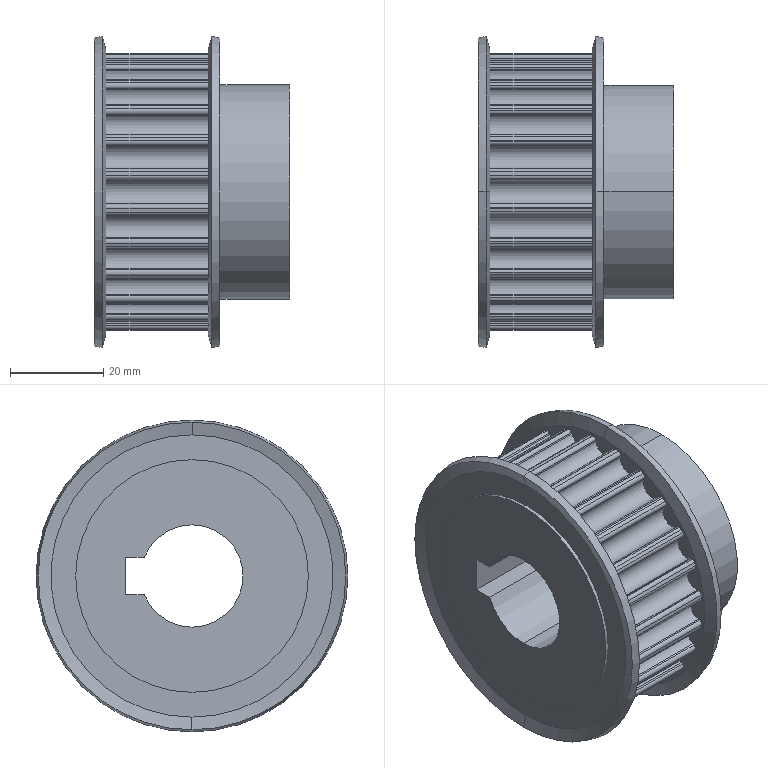Part | STEP file | C-HTPA24H8M200-B-H22 tube-changer main pulley SGN-2-03 | 1 solid | 198 faces | box 42 x 67 x 67 mm | volume 76472 mm3 | cylinder 128 | plane 58 | cone 12 | commonest cylinder face diameters 1.62 x60 5.14 x35 59.74 x24 50 x4 22 x3 46 x2